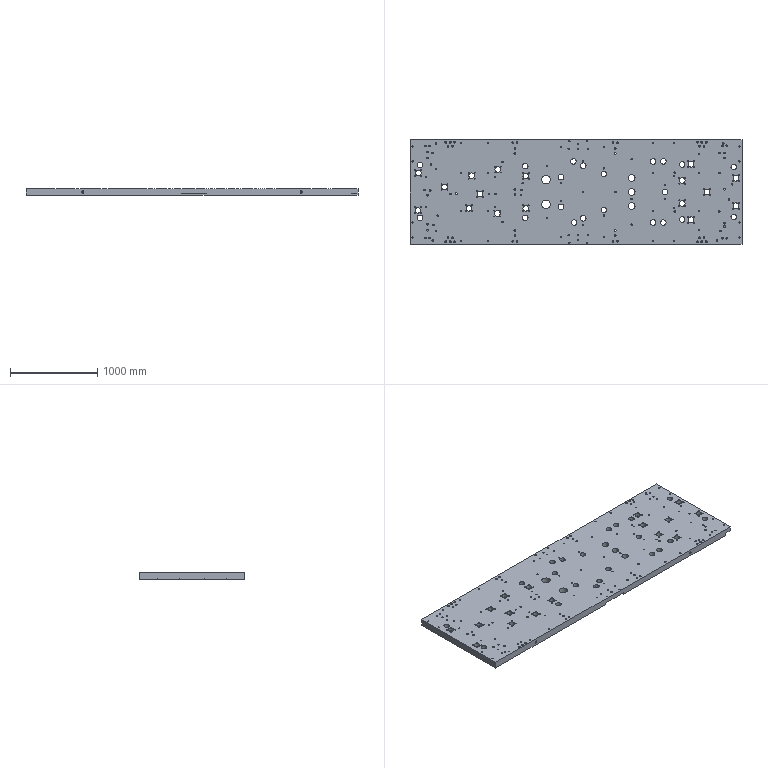Part | STEP file | lll_id6_x_t | 1 solid | 1357 faces | box 3800 x 1200 x 80 mm | volume 344371267 mm3 | cylinder 694 | cone 471 | plane 192 | commonest cylinder face diameters 10.506 x162 14.506 x99 10 x72 6.806 x58 20 x41 17.506 x33